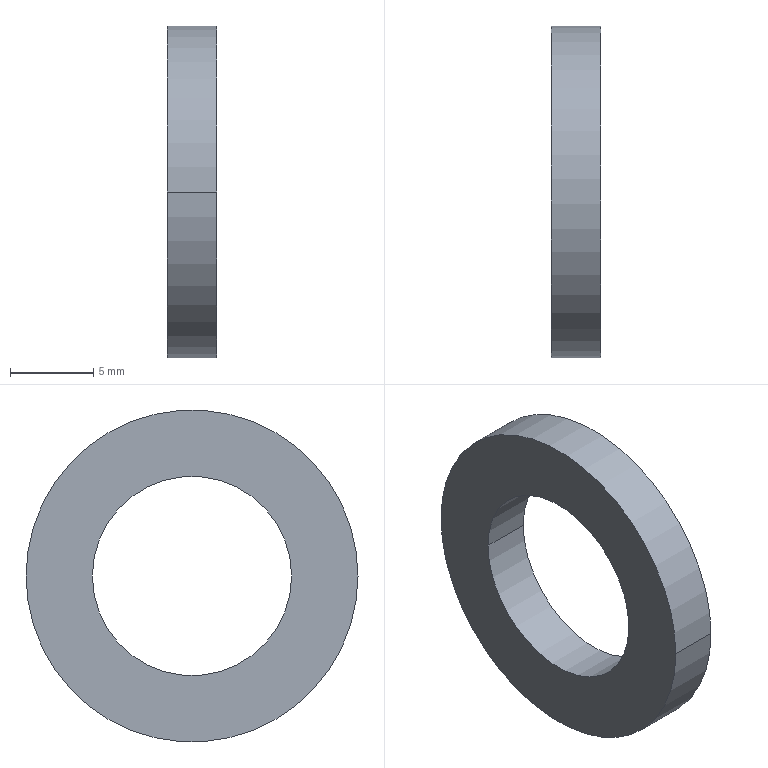Part | STEP file | 0246_005_WSJJ20-12-3 | 1 solid | 6 faces | box 3 x 20 x 20 mm | volume 603.186 mm3 | cylinder 4 | plane 2 | commonest cylinder face diameters 12 x2 20 x2
STEP:
#1=CARTESIAN_POINT('',(0.,0.,0.));
#2=DIRECTION('',(0.,0.,1.));
#3=DIRECTION('',(1.,0.,0.));
#4=AXIS2_PLACEMENT_3D('',#1,#2,#3);
#5=CARTESIAN_POINT('',(3.,10.,0.));
#6=VERTEX_POINT('',#5);
#7=CARTESIAN_POINT('',(3.,-10.,0.));
#8=VERTEX_POINT('',#7);
#9=CARTESIAN_POINT('',(3.,0.,0.));
#10=DIRECTION('',(1.,0.,0.));
#11=DIRECTION('',(0.,-1.,0.));
#12=AXIS2_PLACEMENT_3D('',#9,#10,#11);
#13=CIRCLE('',#12,10.);
#14=CARTESIAN_POINT('',(1.5,0.,0.));
#15=DIRECTION('',(-1.,0.,0.));
#16=DIRECTION('',(0.,-1.,0.));
#17=AXIS2_PLACEMENT_3D('',#14,#15,#16);
#18=CYLINDRICAL_SURFACE('',#17,10.);
#19=CARTESIAN_POINT('',(6.283,-1.5));
#20=DIRECTION('',(-1.,0.));
#21=VECTOR('',#20,1.);
#22=LINE('',#19,#21);
#23=(GEOMETRIC_REPRESENTATION_CONTEXT(2)PARAMETRIC_REPRESENTATION_CONTEXT()REPRESENTATION_CONTEXT('',''));
#24=DEFINITIONAL_REPRESENTATION('',(#22),#23);
#25=PCURVE('',#18,#24);
#26=CARTESIAN_POINT('',(3.,-8.,0.));
#27=DIRECTION('',(1.,0.,0.));
#28=DIRECTION('',(0.,0.,-1.));
#29=AXIS2_PLACEMENT_3D('',#26,#27,#28);
#30=PLANE('',#29);
#31=CARTESIAN_POINT('',(0.,8.));
#32=DIRECTION('',(0.,-1.));
#33=AXIS2_PLACEMENT_2D('',#31,#32);
#34=CIRCLE('',#33,10.);
#35=(GEOMETRIC_REPRESENTATION_CONTEXT(2)PARAMETRIC_REPRESENTATION_CONTEXT()REPRESENTATION_CONTEXT('',''));
#36=DEFINITIONAL_REPRESENTATION('',(#34),#35);
#37=PCURVE('',#30,#36);
#38=SURFACE_CURVE('',#13,(#25,#37),.PCURVE_S1.);
#39=EDGE_CURVE('',#6,#8,#38,.T.);
#40=ORIENTED_EDGE('',*,*,#39,.F.);
#41=CARTESIAN_POINT('',(0.,10.,0.));
#42=VERTEX_POINT('',#41);
#43=CARTESIAN_POINT('',(1.5,10.,0.));
#44=DIRECTION('',(-1.,0.,0.));
#45=VECTOR('',#44,1.);
#46=LINE('',#43,#45);
#47=CARTESIAN_POINT('',(3.142,0.));
#48=DIRECTION('',(0.,1.));
#49=VECTOR('',#48,1.);
#50=LINE('',#47,#49);
#51=(GEOMETRIC_REPRESENTATION_CONTEXT(2)PARAMETRIC_REPRESENTATION_CONTEXT()REPRESENTATION_CONTEXT('',''));
#52=DEFINITIONAL_REPRESENTATION('',(#50),#51);
#53=PCURVE('',#18,#52);
#54=CARTESIAN_POINT('',(1.5,0.,0.));
#55=DIRECTION('',(-1.,0.,0.));
#56=DIRECTION('',(0.,-1.,0.));
#57=AXIS2_PLACEMENT_3D('',#54,#55,#56);
#58=CYLINDRICAL_SURFACE('',#57,10.);
#59=CARTESIAN_POINT('',(3.142,0.));
#60=DIRECTION('',(0.,1.));
#61=VECTOR('',#60,1.);
#62=LINE('',#59,#61);
#63=(GEOMETRIC_REPRESENTATION_CONTEXT(2)PARAMETRIC_REPRESENTATION_CONTEXT()REPRESENTATION_CONTEXT('',''));
#64=DEFINITIONAL_REPRESENTATION('',(#62),#63);
#65=PCURVE('',#58,#64);
#66=SURFACE_CURVE('',#46,(#53,#65),.PCURVE_S1.);
#67=EDGE_CURVE('',#6,#42,#66,.T.);
#68=ORIENTED_EDGE('',*,*,#67,.T.);
#69=CARTESIAN_POINT('',(0.,-10.,0.));
#70=VERTEX_POINT('',#69);
#71=CARTESIAN_POINT('',(0.,0.,0.));
#72=DIRECTION('',(1.,0.,0.));
#73=DIRECTION('',(0.,-1.,0.));
#74=AXIS2_PLACEMENT_3D('',#71,#72,#73);
#75=CIRCLE('',#74,10.);
#76=CARTESIAN_POINT('',(6.283,1.5));
#77=DIRECTION('',(-1.,0.));
#78=VECTOR('',#77,1.);
#79=LINE('',#76,#78);
#80=(GEOMETRIC_REPRESENTATION_CONTEXT(2)PARAMETRIC_REPRESENTATION_CONTEXT()REPRESENTATION_CONTEXT('',''));
#81=DEFINITIONAL_REPRESENTATION('',(#79),#80);
#82=PCURVE('',#18,#81);
#83=CARTESIAN_POINT('',(0.,-8.,0.));
#84=DIRECTION('',(-1.,0.,0.));
#85=DIRECTION('',(0.,-1.,0.));
#86=AXIS2_PLACEMENT_3D('',#83,#84,#85);
#87=PLANE('',#86);
#88=CARTESIAN_POINT('',(2.,0.));
#89=CARTESIAN_POINT('',(2.,-17.321));
#90=CARTESIAN_POINT('',(-13.,-8.66));
#91=CARTESIAN_POINT('',(-28.,0.));
#92=CARTESIAN_POINT('',(-13.,8.66));
#93=CARTESIAN_POINT('',(2.,17.321));
#94=CARTESIAN_POINT('',(2.,0.));
#95=(BOUNDED_CURVE()B_SPLINE_CURVE(2,(#88,#89,#90,#91,#92,#93,#94),.UNSPECIFIED.,.T.,.F.)B_SPLINE_CURVE_WITH_KNOTS((1,2,2,2,2,1),(-2.094,0.,2.094,4.189,6.283,8.378),.UNSPECIFIED.)CURVE()GEOMETRIC_REPRESENTATION_ITEM()RATIONAL_B_SPLINE_CURVE((1.,0.5,1.,0.5,1.,0.5,1.))REPRESENTATION_ITEM(''));
#96=(GEOMETRIC_REPRESENTATION_CONTEXT(2)PARAMETRIC_REPRESENTATION_CONTEXT()REPRESENTATION_CONTEXT('',''));
#97=DEFINITIONAL_REPRESENTATION('',(#95),#96);
#98=PCURVE('',#87,#97);
#99=SURFACE_CURVE('',#75,(#82,#98),.PCURVE_S1.);
#100=EDGE_CURVE('',#42,#70,#99,.T.);
#101=ORIENTED_EDGE('',*,*,#100,.T.);
#102=CARTESIAN_POINT('',(1.5,-10.,0.));
#103=DIRECTION('',(-1.,0.,0.));
#104=VECTOR('',#103,1.);
#105=LINE('',#102,#104);
#106=CARTESIAN_POINT('',(0.,0.));
#107=DIRECTION('',(0.,1.));
#108=VECTOR('',#107,1.);
#109=LINE('',#106,#108);
#110=(GEOMETRIC_REPRESENTATION_CONTEXT(2)PARAMETRIC_REPRESENTATION_CONTEXT()REPRESENTATION_CONTEXT('',''));
#111=DEFINITIONAL_REPRESENTATION('',(#109),#110);
#112=PCURVE('',#18,#111);
#113=CARTESIAN_POINT('',(6.283,0.));
#114=DIRECTION('',(0.,1.));
#115=VECTOR('',#114,1.);
#116=LINE('',#113,#115);
#117=(GEOMETRIC_REPRESENTATION_CONTEXT(2)PARAMETRIC_REPRESENTATION_CONTEXT()REPRESENTATION_CONTEXT('',''));
#118=DEFINITIONAL_REPRESENTATION('',(#116),#117);
#119=PCURVE('',#58,#118);
#120=SURFACE_CURVE('',#105,(#112,#119),.PCURVE_S1.);
#121=EDGE_CURVE('',#8,#70,#120,.T.);
#122=ORIENTED_EDGE('',*,*,#121,.F.);
#123=EDGE_LOOP('',(#40,#68,#101,#122));
#124=FACE_BOUND('',#123,.T.);
#125=ADVANCED_FACE('',(#124),#18,.T.);
#126=CARTESIAN_POINT('',(3.,-6.,0.));
#127=VERTEX_POINT('',#126);
#128=CARTESIAN_POINT('',(0.,-6.,0.));
#129=VERTEX_POINT('',#128);
#130=CARTESIAN_POINT('',(1.5,-6.,0.));
#131=DIRECTION('',(-1.,0.,0.));
#132=VECTOR('',#131,1.);
#133=LINE('',#130,#132);
#134=CARTESIAN_POINT('',(1.5,0.,0.));
#135=DIRECTION('',(-1.,0.,0.));
#136=DIRECTION('',(0.,-1.,0.));
#137=AXIS2_PLACEMENT_3D('',#134,#135,#136);
#138=CYLINDRICAL_SURFACE('',#137,6.);
#139=CARTESIAN_POINT('',(6.283,0.));
#140=DIRECTION('',(0.,1.));
#141=VECTOR('',#140,1.);
#142=LINE('',#139,#141);
#143=(GEOMETRIC_REPRESENTATION_CONTEXT(2)PARAMETRIC_REPRESENTATION_CONTEXT()REPRESENTATION_CONTEXT('',''));
#144=DEFINITIONAL_REPRESENTATION('',(#142),#143);
#145=PCURVE('',#138,#144);
#146=CARTESIAN_POINT('',(1.5,0.,0.));
#147=DIRECTION('',(-1.,0.,0.));
#148=DIRECTION('',(0.,-1.,0.));
#149=AXIS2_PLACEMENT_3D('',#146,#147,#148);
#150=CYLINDRICAL_SURFACE('',#149,6.);
#151=CARTESIAN_POINT('',(0.,0.));
#152=DIRECTION('',(0.,1.));
#153=VECTOR('',#152,1.);
#154=LINE('',#151,#153);
#155=(GEOMETRIC_REPRESENTATION_CONTEXT(2)PARAMETRIC_REPRESENTATION_CONTEXT()REPRESENTATION_CONTEXT('',''));
#156=DEFINITIONAL_REPRESENTATION('',(#154),#155);
#157=PCURVE('',#150,#156);
#158=SURFACE_CURVE('',#133,(#145,#157),.PCURVE_S1.);
#159=EDGE_CURVE('',#127,#129,#158,.T.);
#160=ORIENTED_EDGE('',*,*,#159,.T.);
#161=CARTESIAN_POINT('',(0.,6.,0.));
#162=VERTEX_POINT('',#161);
#163=CARTESIAN_POINT('',(0.,0.,0.));
#164=DIRECTION('',(1.,0.,0.));
#165=DIRECTION('',(0.,-1.,0.));
#166=AXIS2_PLACEMENT_3D('',#163,#164,#165);
#167=CIRCLE('',#166,6.);
#168=CARTESIAN_POINT('',(6.283,1.5));
#169=DIRECTION('',(-1.,0.));
#170=VECTOR('',#169,1.);
#171=LINE('',#168,#170);
#172=(GEOMETRIC_REPRESENTATION_CONTEXT(2)PARAMETRIC_REPRESENTATION_CONTEXT()REPRESENTATION_CONTEXT('',''));
#173=DEFINITIONAL_REPRESENTATION('',(#171),#172);
#174=PCURVE('',#138,#173);
#175=CARTESIAN_POINT('',(-2.,0.));
#176=CARTESIAN_POINT('',(-2.,-10.392));
#177=CARTESIAN_POINT('',(-11.,-5.196));
#178=CARTESIAN_POINT('',(-20.,0.));
#179=CARTESIAN_POINT('',(-11.,5.196));
#180=CARTESIAN_POINT('',(-2.,10.392));
#181=CARTESIAN_POINT('',(-2.,0.));
#182=(BOUNDED_CURVE()B_SPLINE_CURVE(2,(#175,#176,#177,#178,#179,#180,#181),.UNSPECIFIED.,.T.,.F.)B_SPLINE_CURVE_WITH_KNOTS((1,2,2,2,2,1),(-2.094,0.,2.094,4.189,6.283,8.378),.UNSPECIFIED.)CURVE()GEOMETRIC_REPRESENTATION_ITEM()RATIONAL_B_SPLINE_CURVE((1.,0.5,1.,0.5,1.,0.5,1.))REPRESENTATION_ITEM(''));
#183=(GEOMETRIC_REPRESENTATION_CONTEXT(2)PARAMETRIC_REPRESENTATION_CONTEXT()REPRESENTATION_CONTEXT('',''));
#184=DEFINITIONAL_REPRESENTATION('',(#182),#183);
#185=PCURVE('',#87,#184);
#186=SURFACE_CURVE('',#167,(#174,#185),.PCURVE_S1.);
#187=EDGE_CURVE('',#129,#162,#186,.T.);
#188=ORIENTED_EDGE('',*,*,#187,.T.);
#189=CARTESIAN_POINT('',(3.,6.,0.));
#190=VERTEX_POINT('',#189);
#191=CARTESIAN_POINT('',(1.5,6.,0.));
#192=DIRECTION('',(-1.,0.,0.));
#193=VECTOR('',#192,1.);
#194=LINE('',#191,#193);
#195=CARTESIAN_POINT('',(3.142,0.));
#196=DIRECTION('',(0.,1.));
#197=VECTOR('',#196,1.);
#198=LINE('',#195,#197);
#199=(GEOMETRIC_REPRESENTATION_CONTEXT(2)PARAMETRIC_REPRESENTATION_CONTEXT()REPRESENTATION_CONTEXT('',''));
#200=DEFINITIONAL_REPRESENTATION('',(#198),#199);
#201=PCURVE('',#138,#200);
#202=CARTESIAN_POINT('',(3.142,0.));
#203=DIRECTION('',(0.,1.));
#204=VECTOR('',#203,1.);
#205=LINE('',#202,#204);
#206=(GEOMETRIC_REPRESENTATION_CONTEXT(2)PARAMETRIC_REPRESENTATION_CONTEXT()REPRESENTATION_CONTEXT('',''));
#207=DEFINITIONAL_REPRESENTATION('',(#205),#206);
#208=PCURVE('',#150,#207);
#209=SURFACE_CURVE('',#194,(#201,#208),.PCURVE_S1.);
#210=EDGE_CURVE('',#190,#162,#209,.T.);
#211=ORIENTED_EDGE('',*,*,#210,.F.);
#212=CARTESIAN_POINT('',(3.,0.,0.));
#213=DIRECTION('',(-1.,0.,0.));
#214=DIRECTION('',(0.,-1.,0.));
#215=AXIS2_PLACEMENT_3D('',#212,#213,#214);
#216=CIRCLE('',#215,6.);
#217=CARTESIAN_POINT('',(0.,-1.5));
#218=DIRECTION('',(1.,0.));
#219=VECTOR('',#218,1.);
#220=LINE('',#217,#219);
#221=(GEOMETRIC_REPRESENTATION_CONTEXT(2)PARAMETRIC_REPRESENTATION_CONTEXT()REPRESENTATION_CONTEXT('',''));
#222=DEFINITIONAL_REPRESENTATION('',(#220),#221);
#223=PCURVE('',#138,#222);
#224=CARTESIAN_POINT('',(0.,2.));
#225=CARTESIAN_POINT('',(-10.392,2.));
#226=CARTESIAN_POINT('',(-5.196,11.));
#227=CARTESIAN_POINT('',(0.,20.));
#228=CARTESIAN_POINT('',(5.196,11.));
#229=CARTESIAN_POINT('',(10.392,2.));
#230=CARTESIAN_POINT('',(0.,2.));
#231=(BOUNDED_CURVE()B_SPLINE_CURVE(2,(#224,#225,#226,#227,#228,#229,#230),.UNSPECIFIED.,.T.,.F.)B_SPLINE_CURVE_WITH_KNOTS((1,2,2,2,2,1),(-2.094,0.,2.094,4.189,6.283,8.378),.UNSPECIFIED.)CURVE()GEOMETRIC_REPRESENTATION_ITEM()RATIONAL_B_SPLINE_CURVE((1.,0.5,1.,0.5,1.,0.5,1.))REPRESENTATION_ITEM(''));
#232=(GEOMETRIC_REPRESENTATION_CONTEXT(2)PARAMETRIC_REPRESENTATION_CONTEXT()REPRESENTATION_CONTEXT('',''));
#233=DEFINITIONAL_REPRESENTATION('',(#231),#232);
#234=PCURVE('',#30,#233);
#235=SURFACE_CURVE('',#216,(#223,#234),.PCURVE_S1.);
#236=EDGE_CURVE('',#190,#127,#235,.T.);
#237=ORIENTED_EDGE('',*,*,#236,.T.);
#238=EDGE_LOOP('',(#160,#188,#211,#237));
#239=FACE_BOUND('',#238,.F.);
#240=ADVANCED_FACE('',(#239),#138,.F.);
#241=CARTESIAN_POINT('',(3.,0.,0.));
#242=DIRECTION('',(1.,0.,0.));
#243=DIRECTION('',(0.,-1.,0.));
#244=AXIS2_PLACEMENT_3D('',#241,#242,#243);
#245=CIRCLE('',#244,10.);
#246=CARTESIAN_POINT('',(0.,8.));
#247=DIRECTION('',(0.,-1.));
#248=AXIS2_PLACEMENT_2D('',#246,#247);
#249=CIRCLE('',#248,10.);
#250=(GEOMETRIC_REPRESENTATION_CONTEXT(2)PARAMETRIC_REPRESENTATION_CONTEXT()REPRESENTATION_CONTEXT('',''));
#251=DEFINITIONAL_REPRESENTATION('',(#249),#250);
#252=PCURVE('',#30,#251);
#253=CARTESIAN_POINT('',(6.283,-1.5));
#254=DIRECTION('',(-1.,0.));
#255=VECTOR('',#254,1.);
#256=LINE('',#253,#255);
#257=(GEOMETRIC_REPRESENTATION_CONTEXT(2)PARAMETRIC_REPRESENTATION_CONTEXT()REPRESENTATION_CONTEXT('',''));
#258=DEFINITIONAL_REPRESENTATION('',(#256),#257);
#259=PCURVE('',#58,#258);
#260=SURFACE_CURVE('',#245,(#252,#259),.PCURVE_S1.);
#261=EDGE_CURVE('',#8,#6,#260,.T.);
#262=ORIENTED_EDGE('',*,*,#261,.T.);
#263=ORIENTED_EDGE('',*,*,#39,.T.);
#264=EDGE_LOOP('',(#262,#263));
#265=FACE_BOUND('',#264,.T.);
#266=CARTESIAN_POINT('',(3.,0.,0.));
#267=DIRECTION('',(-1.,0.,0.));
#268=DIRECTION('',(0.,-1.,0.));
#269=AXIS2_PLACEMENT_3D('',#266,#267,#268);
#270=CIRCLE('',#269,6.);
#271=CARTESIAN_POINT('',(0.,2.));
#272=CARTESIAN_POINT('',(-10.392,2.));
#273=CARTESIAN_POINT('',(-5.196,11.));
#274=CARTESIAN_POINT('',(0.,20.));
#275=CARTESIAN_POINT('',(5.196,11.));
#276=CARTESIAN_POINT('',(10.392,2.));
#277=CARTESIAN_POINT('',(0.,2.));
#278=(BOUNDED_CURVE()B_SPLINE_CURVE(2,(#271,#272,#273,#274,#275,#276,#277),.UNSPECIFIED.,.T.,.F.)B_SPLINE_CURVE_WITH_KNOTS((1,2,2,2,2,1),(-2.094,0.,2.094,4.189,6.283,8.378),.UNSPECIFIED.)CURVE()GEOMETRIC_REPRESENTATION_ITEM()RATIONAL_B_SPLINE_CURVE((1.,0.5,1.,0.5,1.,0.5,1.))REPRESENTATION_ITEM(''));
#279=(GEOMETRIC_REPRESENTATION_CONTEXT(2)PARAMETRIC_REPRESENTATION_CONTEXT()REPRESENTATION_CONTEXT('',''));
#280=DEFINITIONAL_REPRESENTATION('',(#278),#279);
#281=PCURVE('',#30,#280);
#282=CARTESIAN_POINT('',(0.,-1.5));
#283=DIRECTION('',(1.,0.));
#284=VECTOR('',#283,1.);
#285=LINE('',#282,#284);
#286=(GEOMETRIC_REPRESENTATION_CONTEXT(2)PARAMETRIC_REPRESENTATION_CONTEXT()REPRESENTATION_CONTEXT('',''));
#287=DEFINITIONAL_REPRESENTATION('',(#285),#286);
#288=PCURVE('',#150,#287);
#289=SURFACE_CURVE('',#270,(#281,#288),.PCURVE_S1.);
#290=EDGE_CURVE('',#127,#190,#289,.T.);
#291=ORIENTED_EDGE('',*,*,#290,.T.);
#292=ORIENTED_EDGE('',*,*,#236,.T.);
#293=EDGE_LOOP('',(#291,#292));
#294=FACE_BOUND('',#293,.T.);
#295=ADVANCED_FACE('',(#265,#294),#30,.T.);
#296=ORIENTED_EDGE('',*,*,#67,.F.);
#297=ORIENTED_EDGE('',*,*,#261,.F.);
#298=ORIENTED_EDGE('',*,*,#121,.T.);
#299=CARTESIAN_POINT('',(0.,0.,0.));
#300=DIRECTION('',(1.,0.,0.));
#301=DIRECTION('',(0.,-1.,0.));
#302=AXIS2_PLACEMENT_3D('',#299,#300,#301);
#303=CIRCLE('',#302,10.);
#304=CARTESIAN_POINT('',(6.283,1.5));
#305=DIRECTION('',(-1.,0.));
#306=VECTOR('',#305,1.);
#307=LINE('',#304,#306);
#308=(GEOMETRIC_REPRESENTATION_CONTEXT(2)PARAMETRIC_REPRESENTATION_CONTEXT()REPRESENTATION_CONTEXT('',''));
#309=DEFINITIONAL_REPRESENTATION('',(#307),#308);
#310=PCURVE('',#58,#309);
#311=CARTESIAN_POINT('',(2.,0.));
#312=CARTESIAN_POINT('',(2.,-17.321));
#313=CARTESIAN_POINT('',(-13.,-8.66));
#314=CARTESIAN_POINT('',(-28.,0.));
#315=CARTESIAN_POINT('',(-13.,8.66));
#316=CARTESIAN_POINT('',(2.,17.321));
#317=CARTESIAN_POINT('',(2.,0.));
#318=(BOUNDED_CURVE()B_SPLINE_CURVE(2,(#311,#312,#313,#314,#315,#316,#317),.UNSPECIFIED.,.T.,.F.)B_SPLINE_CURVE_WITH_KNOTS((1,2,2,2,2,1),(-2.094,0.,2.094,4.189,6.283,8.378),.UNSPECIFIED.)CURVE()GEOMETRIC_REPRESENTATION_ITEM()RATIONAL_B_SPLINE_CURVE((1.,0.5,1.,0.5,1.,0.5,1.))REPRESENTATION_ITEM(''));
#319=(GEOMETRIC_REPRESENTATION_CONTEXT(2)PARAMETRIC_REPRESENTATION_CONTEXT()REPRESENTATION_CONTEXT('',''));
#320=DEFINITIONAL_REPRESENTATION('',(#318),#319);
#321=PCURVE('',#87,#320);
#322=SURFACE_CURVE('',#303,(#310,#321),.PCURVE_S1.);
#323=EDGE_CURVE('',#70,#42,#322,.T.);
#324=ORIENTED_EDGE('',*,*,#323,.T.);
#325=EDGE_LOOP('',(#296,#297,#298,#324));
#326=FACE_BOUND('',#325,.T.);
#327=ADVANCED_FACE('',(#326),#58,.T.);
#328=CARTESIAN_POINT('',(0.,0.,0.));
#329=DIRECTION('',(1.,0.,0.));
#330=DIRECTION('',(0.,-1.,0.));
#331=AXIS2_PLACEMENT_3D('',#328,#329,#330);
#332=CIRCLE('',#331,6.);
#333=CARTESIAN_POINT('',(6.283,1.5));
#334=DIRECTION('',(-1.,0.));
#335=VECTOR('',#334,1.);
#336=LINE('',#333,#335);
#337=(GEOMETRIC_REPRESENTATION_CONTEXT(2)PARAMETRIC_REPRESENTATION_CONTEXT()REPRESENTATION_CONTEXT('',''));
#338=DEFINITIONAL_REPRESENTATION('',(#336),#337);
#339=PCURVE('',#150,#338);
#340=CARTESIAN_POINT('',(-2.,0.));
#341=CARTESIAN_POINT('',(-2.,-10.392));
#342=CARTESIAN_POINT('',(-11.,-5.196));
#343=CARTESIAN_POINT('',(-20.,0.));
#344=CARTESIAN_POINT('',(-11.,5.196));
#345=CARTESIAN_POINT('',(-2.,10.392));
#346=CARTESIAN_POINT('',(-2.,0.));
#347=(BOUNDED_CURVE()B_SPLINE_CURVE(2,(#340,#341,#342,#343,#344,#345,#346),.UNSPECIFIED.,.T.,.F.)B_SPLINE_CURVE_WITH_KNOTS((1,2,2,2,2,1),(-2.094,0.,2.094,4.189,6.283,8.378),.UNSPECIFIED.)CURVE()GEOMETRIC_REPRESENTATION_ITEM()RATIONAL_B_SPLINE_CURVE((1.,0.5,1.,0.5,1.,0.5,1.))REPRESENTATION_ITEM(''));
#348=(GEOMETRIC_REPRESENTATION_CONTEXT(2)PARAMETRIC_REPRESENTATION_CONTEXT()REPRESENTATION_CONTEXT('',''));
#349=DEFINITIONAL_REPRESENTATION('',(#347),#348);
#350=PCURVE('',#87,#349);
#351=SURFACE_CURVE('',#332,(#339,#350),.PCURVE_S1.);
#352=EDGE_CURVE('',#162,#129,#351,.T.);
#353=ORIENTED_EDGE('',*,*,#352,.T.);
#354=ORIENTED_EDGE('',*,*,#159,.F.);
#355=ORIENTED_EDGE('',*,*,#290,.T.);
#356=ORIENTED_EDGE('',*,*,#210,.T.);
#357=EDGE_LOOP('',(#353,#354,#355,#356));
#358=FACE_BOUND('',#357,.F.);
#359=ADVANCED_FACE('',(#358),#150,.F.);
#360=ORIENTED_EDGE('',*,*,#187,.T.);
#361=ORIENTED_EDGE('',*,*,#352,.T.);
#362=EDGE_LOOP('',(#360,#361));
#363=FACE_BOUND('',#362,.T.);
#364=ORIENTED_EDGE('',*,*,#323,.F.);
#365=ORIENTED_EDGE('',*,*,#100,.F.);
#366=EDGE_LOOP('',(#364,#365));
#367=FACE_BOUND('',#366,.T.);
#368=ADVANCED_FACE('',(#363,#367),#87,.T.);
#369=CLOSED_SHELL('',(#125,#240,#295,#327,#359,#368));
#370=MANIFOLD_SOLID_BREP('',#369);
#371=(LENGTH_UNIT()NAMED_UNIT(*)SI_UNIT(.MILLI.,.METRE.));
#372=UNCERTAINTY_MEASURE_WITH_UNIT(LENGTH_MEASURE(0.0000001),#371,'','');
#373=(NAMED_UNIT(*)PLANE_ANGLE_UNIT()SI_UNIT($,.RADIAN.));
#374=(NAMED_UNIT(*)SI_UNIT($,.STERADIAN.)SOLID_ANGLE_UNIT());
#375=(GEOMETRIC_REPRESENTATION_CONTEXT(3)GLOBAL_UNCERTAINTY_ASSIGNED_CONTEXT((#372))GLOBAL_UNIT_ASSIGNED_CONTEXT((#371,#373,#374))REPRESENTATION_CONTEXT('',''));
#376=ADVANCED_BREP_SHAPE_REPRESENTATION('',(#4,#370),#375);